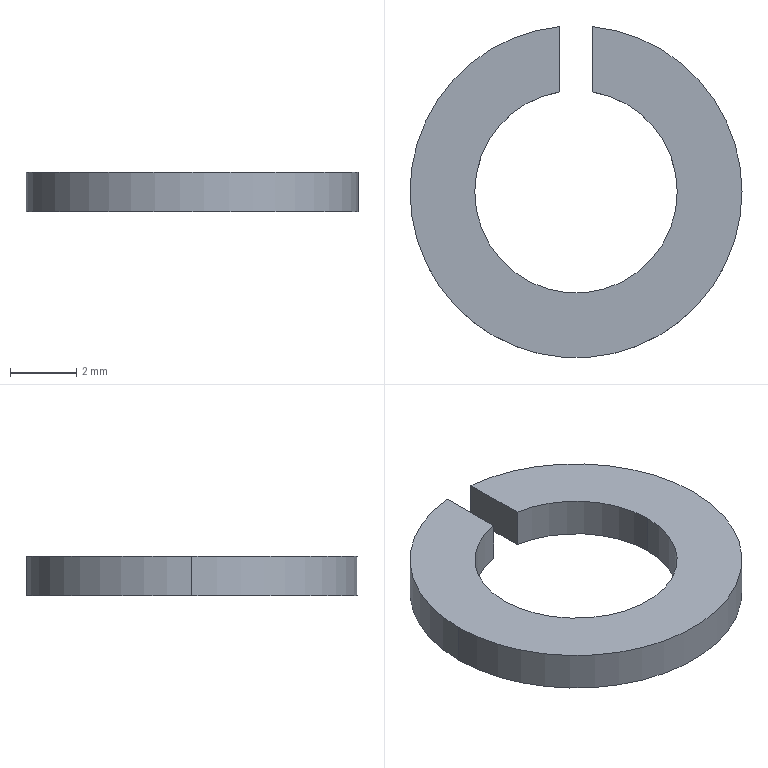Part | SolidWorks | features Extrusion 1 | 1 solid | 10 faces | box 10 x 9.975 x 1.2 mm | volume 56.832 mm3 | cylinder 6 | plane 4 | commonest cylinder face diameters 6.1 x3 10 x3
STEP:
#1=CARTESIAN_POINT('',(3.05,0.,228.7));
#2=VERTEX_POINT('',#1);
#3=CARTESIAN_POINT('',(-3.05,0.,228.7));
#4=VERTEX_POINT('',#3);
#5=CARTESIAN_POINT('',(0.,0.,228.7));
#6=DIRECTION('',(0.,0.,-1.));
#7=DIRECTION('',(-1.,0.,0.));
#8=AXIS2_PLACEMENT_3D('',#5,#6,#7);
#9=CIRCLE('',#8,3.05);
#10=EDGE_CURVE('',#2,#4,#9,.T.);
#11=ORIENTED_EDGE('',*,*,#10,.T.);
#12=CARTESIAN_POINT('',(-3.05,0.,229.9));
#13=VERTEX_POINT('',#12);
#14=CARTESIAN_POINT('',(-3.05,0.,228.7));
#15=DIRECTION('',(0.,0.,1.));
#16=VECTOR('',#15,1000.);
#17=LINE('',#14,#16);
#18=EDGE_CURVE('',#4,#13,#17,.T.);
#19=ORIENTED_EDGE('',*,*,#18,.T.);
#20=CARTESIAN_POINT('',(3.05,0.,229.9));
#21=VERTEX_POINT('',#20);
#22=CARTESIAN_POINT('',(0.,0.,229.9));
#23=DIRECTION('',(0.,0.,-1.));
#24=DIRECTION('',(-1.,0.,0.));
#25=AXIS2_PLACEMENT_3D('',#22,#23,#24);
#26=CIRCLE('',#25,3.05);
#27=EDGE_CURVE('',#21,#13,#26,.T.);
#28=ORIENTED_EDGE('',*,*,#27,.F.);
#29=CARTESIAN_POINT('',(3.05,0.,228.7));
#30=DIRECTION('',(0.,0.,1.));
#31=VECTOR('',#30,1000.);
#32=LINE('',#29,#31);
#33=EDGE_CURVE('',#2,#21,#32,.T.);
#34=ORIENTED_EDGE('',*,*,#33,.F.);
#35=EDGE_LOOP('',(#11,#19,#28,#34));
#36=FACE_OUTER_BOUND('',#35,.T.);
#37=CARTESIAN_POINT('',(0.,0.,228.7));
#38=DIRECTION('',(0.,0.,1.));
#39=DIRECTION('',(1.,0.,0.));
#40=AXIS2_PLACEMENT_3D('',#37,#38,#39);
#41=CYLINDRICAL_SURFACE('',#40,3.05);
#42=ADVANCED_FACE('',(#36),#41,.F.);
#43=CARTESIAN_POINT('',(0.5,3.009,228.7));
#44=VERTEX_POINT('',#43);
#45=CARTESIAN_POINT('',(0.,0.,228.7));
#46=DIRECTION('',(0.,0.,-1.));
#47=DIRECTION('',(-1.,0.,0.));
#48=AXIS2_PLACEMENT_3D('',#45,#46,#47);
#49=CIRCLE('',#48,3.05);
#50=EDGE_CURVE('',#44,#2,#49,.T.);
#51=ORIENTED_EDGE('',*,*,#50,.T.);
#52=ORIENTED_EDGE('',*,*,#33,.T.);
#53=CARTESIAN_POINT('',(0.5,3.009,229.9));
#54=VERTEX_POINT('',#53);
#55=CARTESIAN_POINT('',(0.,0.,229.9));
#56=DIRECTION('',(0.,0.,-1.));
#57=DIRECTION('',(-1.,0.,0.));
#58=AXIS2_PLACEMENT_3D('',#55,#56,#57);
#59=CIRCLE('',#58,3.05);
#60=EDGE_CURVE('',#54,#21,#59,.T.);
#61=ORIENTED_EDGE('',*,*,#60,.F.);
#62=CARTESIAN_POINT('',(0.5,3.009,228.7));
#63=DIRECTION('',(0.,0.,1.));
#64=VECTOR('',#63,1000.);
#65=LINE('',#62,#64);
#66=EDGE_CURVE('',#44,#54,#65,.T.);
#67=ORIENTED_EDGE('',*,*,#66,.F.);
#68=EDGE_LOOP('',(#51,#52,#61,#67));
#69=FACE_OUTER_BOUND('',#68,.T.);
#70=CARTESIAN_POINT('',(0.,0.,228.7));
#71=DIRECTION('',(0.,0.,1.));
#72=DIRECTION('',(1.,0.,0.));
#73=AXIS2_PLACEMENT_3D('',#70,#71,#72);
#74=CYLINDRICAL_SURFACE('',#73,3.05);
#75=ADVANCED_FACE('',(#69),#74,.F.);
#76=CARTESIAN_POINT('',(-0.5,4.975,228.7));
#77=VERTEX_POINT('',#76);
#78=CARTESIAN_POINT('',(-5.,0.,228.7));
#79=VERTEX_POINT('',#78);
#80=CARTESIAN_POINT('',(0.,0.,228.7));
#81=DIRECTION('',(0.,0.,1.));
#82=DIRECTION('',(1.,0.,0.));
#83=AXIS2_PLACEMENT_3D('',#80,#81,#82);
#84=CIRCLE('',#83,5.);
#85=EDGE_CURVE('',#77,#79,#84,.T.);
#86=ORIENTED_EDGE('',*,*,#85,.T.);
#87=CARTESIAN_POINT('',(-5.,0.,229.9));
#88=VERTEX_POINT('',#87);
#89=CARTESIAN_POINT('',(-5.,0.,228.7));
#90=DIRECTION('',(0.,0.,1.));
#91=VECTOR('',#90,1000.);
#92=LINE('',#89,#91);
#93=EDGE_CURVE('',#79,#88,#92,.T.);
#94=ORIENTED_EDGE('',*,*,#93,.T.);
#95=CARTESIAN_POINT('',(-0.5,4.975,229.9));
#96=VERTEX_POINT('',#95);
#97=CARTESIAN_POINT('',(0.,0.,229.9));
#98=DIRECTION('',(0.,0.,1.));
#99=DIRECTION('',(1.,0.,0.));
#100=AXIS2_PLACEMENT_3D('',#97,#98,#99);
#101=CIRCLE('',#100,5.);
#102=EDGE_CURVE('',#96,#88,#101,.T.);
#103=ORIENTED_EDGE('',*,*,#102,.F.);
#104=CARTESIAN_POINT('',(-0.5,4.975,228.7));
#105=DIRECTION('',(0.,0.,1.));
#106=VECTOR('',#105,1000.);
#107=LINE('',#104,#106);
#108=EDGE_CURVE('',#77,#96,#107,.T.);
#109=ORIENTED_EDGE('',*,*,#108,.F.);
#110=EDGE_LOOP('',(#86,#94,#103,#109));
#111=FACE_OUTER_BOUND('',#110,.T.);
#112=CARTESIAN_POINT('',(0.,0.,228.7));
#113=DIRECTION('',(0.,0.,1.));
#114=DIRECTION('',(1.,0.,0.));
#115=AXIS2_PLACEMENT_3D('',#112,#113,#114);
#116=CYLINDRICAL_SURFACE('',#115,5.);
#117=ADVANCED_FACE('',(#111),#116,.T.);
#118=ORIENTED_EDGE('',*,*,#93,.F.);
#119=CARTESIAN_POINT('',(5.,0.,228.7));
#120=VERTEX_POINT('',#119);
#121=CARTESIAN_POINT('',(0.,0.,228.7));
#122=DIRECTION('',(0.,0.,1.));
#123=DIRECTION('',(1.,0.,0.));
#124=AXIS2_PLACEMENT_3D('',#121,#122,#123);
#125=CIRCLE('',#124,5.);
#126=EDGE_CURVE('',#79,#120,#125,.T.);
#127=ORIENTED_EDGE('',*,*,#126,.T.);
#128=CARTESIAN_POINT('',(5.,0.,229.9));
#129=VERTEX_POINT('',#128);
#130=CARTESIAN_POINT('',(5.,0.,228.7));
#131=DIRECTION('',(0.,0.,1.));
#132=VECTOR('',#131,1000.);
#133=LINE('',#130,#132);
#134=EDGE_CURVE('',#120,#129,#133,.T.);
#135=ORIENTED_EDGE('',*,*,#134,.T.);
#136=CARTESIAN_POINT('',(0.,0.,229.9));
#137=DIRECTION('',(0.,0.,1.));
#138=DIRECTION('',(1.,0.,0.));
#139=AXIS2_PLACEMENT_3D('',#136,#137,#138);
#140=CIRCLE('',#139,5.);
#141=EDGE_CURVE('',#88,#129,#140,.T.);
#142=ORIENTED_EDGE('',*,*,#141,.F.);
#143=EDGE_LOOP('',(#118,#127,#135,#142));
#144=FACE_OUTER_BOUND('',#143,.T.);
#145=CARTESIAN_POINT('',(0.,0.,228.7));
#146=DIRECTION('',(0.,0.,1.));
#147=DIRECTION('',(1.,0.,0.));
#148=AXIS2_PLACEMENT_3D('',#145,#146,#147);
#149=CYLINDRICAL_SURFACE('',#148,5.);
#150=ADVANCED_FACE('',(#144),#149,.T.);
#151=ORIENTED_EDGE('',*,*,#134,.F.);
#152=CARTESIAN_POINT('',(0.5,4.975,228.7));
#153=VERTEX_POINT('',#152);
#154=CARTESIAN_POINT('',(0.,0.,228.7));
#155=DIRECTION('',(0.,0.,1.));
#156=DIRECTION('',(1.,0.,0.));
#157=AXIS2_PLACEMENT_3D('',#154,#155,#156);
#158=CIRCLE('',#157,5.);
#159=EDGE_CURVE('',#120,#153,#158,.T.);
#160=ORIENTED_EDGE('',*,*,#159,.T.);
#161=CARTESIAN_POINT('',(0.5,4.975,229.9));
#162=VERTEX_POINT('',#161);
#163=CARTESIAN_POINT('',(0.5,4.975,228.7));
#164=DIRECTION('',(0.,0.,1.));
#165=VECTOR('',#164,1000.);
#166=LINE('',#163,#165);
#167=EDGE_CURVE('',#153,#162,#166,.T.);
#168=ORIENTED_EDGE('',*,*,#167,.T.);
#169=CARTESIAN_POINT('',(0.,0.,229.9));
#170=DIRECTION('',(0.,0.,1.));
#171=DIRECTION('',(1.,0.,0.));
#172=AXIS2_PLACEMENT_3D('',#169,#170,#171);
#173=CIRCLE('',#172,5.);
#174=EDGE_CURVE('',#129,#162,#173,.T.);
#175=ORIENTED_EDGE('',*,*,#174,.F.);
#176=EDGE_LOOP('',(#151,#160,#168,#175));
#177=FACE_OUTER_BOUND('',#176,.T.);
#178=CARTESIAN_POINT('',(0.,0.,228.7));
#179=DIRECTION('',(0.,0.,1.));
#180=DIRECTION('',(1.,0.,0.));
#181=AXIS2_PLACEMENT_3D('',#178,#179,#180);
#182=CYLINDRICAL_SURFACE('',#181,5.);
#183=ADVANCED_FACE('',(#177),#182,.T.);
#184=CARTESIAN_POINT('',(-0.5,3.009,229.9));
#185=VERTEX_POINT('',#184);
#186=CARTESIAN_POINT('',(-0.5,3.009,229.9));
#187=DIRECTION('',(0.,1.,0.));
#188=VECTOR('',#187,1000.);
#189=LINE('',#186,#188);
#190=EDGE_CURVE('',#185,#96,#189,.T.);
#191=ORIENTED_EDGE('',*,*,#190,.F.);
#192=CARTESIAN_POINT('',(-0.5,3.009,228.7));
#193=VERTEX_POINT('',#192);
#194=CARTESIAN_POINT('',(-0.5,3.009,228.7));
#195=DIRECTION('',(0.,0.,1.));
#196=VECTOR('',#195,1000.);
#197=LINE('',#194,#196);
#198=EDGE_CURVE('',#193,#185,#197,.T.);
#199=ORIENTED_EDGE('',*,*,#198,.F.);
#200=CARTESIAN_POINT('',(-0.5,3.009,228.7));
#201=DIRECTION('',(0.,1.,0.));
#202=VECTOR('',#201,1000.);
#203=LINE('',#200,#202);
#204=EDGE_CURVE('',#193,#77,#203,.T.);
#205=ORIENTED_EDGE('',*,*,#204,.T.);
#206=ORIENTED_EDGE('',*,*,#108,.T.);
#207=EDGE_LOOP('',(#191,#199,#205,#206));
#208=FACE_OUTER_BOUND('',#207,.T.);
#209=CARTESIAN_POINT('',(-0.5,3.009,228.7));
#210=DIRECTION('',(1.,0.,0.));
#211=DIRECTION('',(0.,0.,-1.));
#212=AXIS2_PLACEMENT_3D('',#209,#210,#211);
#213=PLANE('',#212);
#214=ADVANCED_FACE('',(#208),#213,.T.);
#215=ORIENTED_EDGE('',*,*,#18,.F.);
#216=CARTESIAN_POINT('',(0.,0.,228.7));
#217=DIRECTION('',(0.,0.,-1.));
#218=DIRECTION('',(-1.,0.,0.));
#219=AXIS2_PLACEMENT_3D('',#216,#217,#218);
#220=CIRCLE('',#219,3.05);
#221=EDGE_CURVE('',#4,#193,#220,.T.);
#222=ORIENTED_EDGE('',*,*,#221,.T.);
#223=ORIENTED_EDGE('',*,*,#198,.T.);
#224=CARTESIAN_POINT('',(0.,0.,229.9));
#225=DIRECTION('',(0.,0.,-1.));
#226=DIRECTION('',(-1.,0.,0.));
#227=AXIS2_PLACEMENT_3D('',#224,#225,#226);
#228=CIRCLE('',#227,3.05);
#229=EDGE_CURVE('',#13,#185,#228,.T.);
#230=ORIENTED_EDGE('',*,*,#229,.F.);
#231=EDGE_LOOP('',(#215,#222,#223,#230));
#232=FACE_OUTER_BOUND('',#231,.T.);
#233=CARTESIAN_POINT('',(0.,0.,228.7));
#234=DIRECTION('',(0.,0.,1.));
#235=DIRECTION('',(1.,0.,0.));
#236=AXIS2_PLACEMENT_3D('',#233,#234,#235);
#237=CYLINDRICAL_SURFACE('',#236,3.05);
#238=ADVANCED_FACE('',(#232),#237,.F.);
#239=CARTESIAN_POINT('',(0.5,4.975,229.9));
#240=DIRECTION('',(0.,-1.,0.));
#241=VECTOR('',#240,1000.);
#242=LINE('',#239,#241);
#243=EDGE_CURVE('',#162,#54,#242,.T.);
#244=ORIENTED_EDGE('',*,*,#243,.F.);
#245=ORIENTED_EDGE('',*,*,#167,.F.);
#246=CARTESIAN_POINT('',(0.5,4.975,228.7));
#247=DIRECTION('',(0.,-1.,0.));
#248=VECTOR('',#247,1000.);
#249=LINE('',#246,#248);
#250=EDGE_CURVE('',#153,#44,#249,.T.);
#251=ORIENTED_EDGE('',*,*,#250,.T.);
#252=ORIENTED_EDGE('',*,*,#66,.T.);
#253=EDGE_LOOP('',(#244,#245,#251,#252));
#254=FACE_OUTER_BOUND('',#253,.T.);
#255=CARTESIAN_POINT('',(0.5,4.975,228.7));
#256=DIRECTION('',(-1.,0.,0.));
#257=DIRECTION('',(0.,0.,1.));
#258=AXIS2_PLACEMENT_3D('',#255,#256,#257);
#259=PLANE('',#258);
#260=ADVANCED_FACE('',(#254),#259,.T.);
#261=ORIENTED_EDGE('',*,*,#85,.F.);
#262=ORIENTED_EDGE('',*,*,#204,.F.);
#263=ORIENTED_EDGE('',*,*,#221,.F.);
#264=ORIENTED_EDGE('',*,*,#10,.F.);
#265=ORIENTED_EDGE('',*,*,#50,.F.);
#266=ORIENTED_EDGE('',*,*,#250,.F.);
#267=ORIENTED_EDGE('',*,*,#159,.F.);
#268=ORIENTED_EDGE('',*,*,#126,.F.);
#269=EDGE_LOOP('',(#261,#262,#263,#264,#265,#266,#267,#268));
#270=FACE_OUTER_BOUND('',#269,.T.);
#271=CARTESIAN_POINT('',(0.,0.,228.7));
#272=DIRECTION('',(0.,0.,1.));
#273=DIRECTION('',(1.,0.,0.));
#274=AXIS2_PLACEMENT_3D('',#271,#272,#273);
#275=PLANE('',#274);
#276=ADVANCED_FACE('',(#270),#275,.F.);
#277=ORIENTED_EDGE('',*,*,#102,.T.);
#278=ORIENTED_EDGE('',*,*,#141,.T.);
#279=ORIENTED_EDGE('',*,*,#174,.T.);
#280=ORIENTED_EDGE('',*,*,#243,.T.);
#281=ORIENTED_EDGE('',*,*,#60,.T.);
#282=ORIENTED_EDGE('',*,*,#27,.T.);
#283=ORIENTED_EDGE('',*,*,#229,.T.);
#284=ORIENTED_EDGE('',*,*,#190,.T.);
#285=EDGE_LOOP('',(#277,#278,#279,#280,#281,#282,#283,#284));
#286=FACE_OUTER_BOUND('',#285,.T.);
#287=CARTESIAN_POINT('',(0.,0.,229.9));
#288=DIRECTION('',(0.,0.,1.));
#289=DIRECTION('',(1.,0.,0.));
#290=AXIS2_PLACEMENT_3D('',#287,#288,#289);
#291=PLANE('',#290);
#292=ADVANCED_FACE('',(#286),#291,.T.);
#293=CLOSED_SHELL('',(#42,#75,#117,#150,#183,#214,#238,#260,#276,#292));
#294=MANIFOLD_SOLID_BREP('',#293);
#295=CARTESIAN_POINT('',(0.,0.,0.));
#296=DIRECTION('',(0.,0.,1.));
#297=DIRECTION('',(1.,0.,0.));
#298=AXIS2_PLACEMENT_3D('',#295,#296,#297);
#299=(LENGTH_UNIT()NAMED_UNIT(*)SI_UNIT(.MILLI.,.METRE.));
#300=UNCERTAINTY_MEASURE_WITH_UNIT(LENGTH_MEASURE(0.00001),#299,'','');
#301=(NAMED_UNIT(*)PLANE_ANGLE_UNIT()SI_UNIT($,.RADIAN.));
#302=(NAMED_UNIT(*)SI_UNIT($,.STERADIAN.)SOLID_ANGLE_UNIT());
#303=(GEOMETRIC_REPRESENTATION_CONTEXT(3)GLOBAL_UNCERTAINTY_ASSIGNED_CONTEXT((#300))GLOBAL_UNIT_ASSIGNED_CONTEXT((#299,#301,#302))REPRESENTATION_CONTEXT('',''));
#304=ADVANCED_BREP_SHAPE_REPRESENTATION('',(#294,#298),#303);